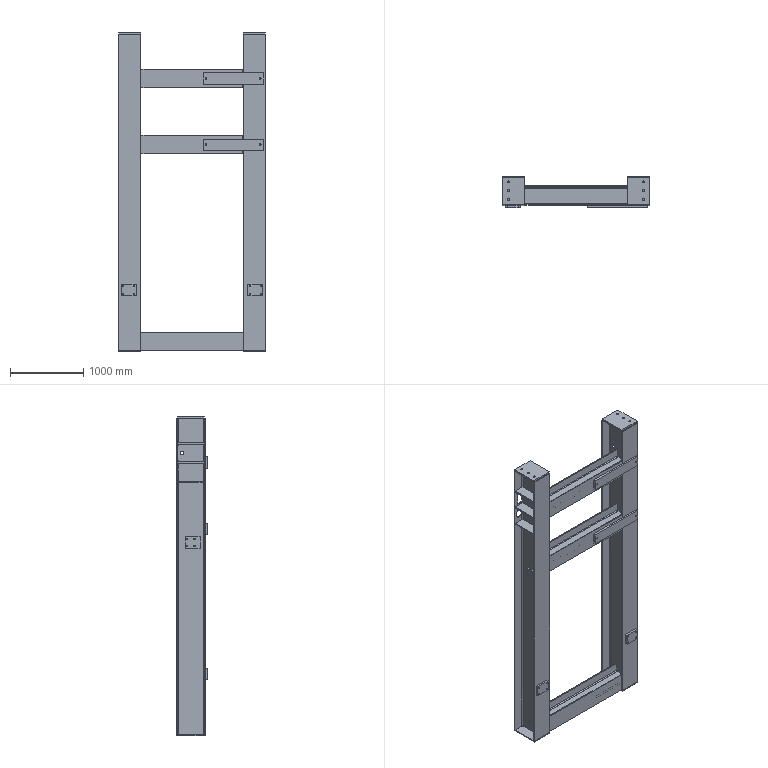Part | SolidWorks | 20 solids | 262 faces | box 1990 x 420 x 4350 mm | volume 182192599 mm3 | plane 187 | cylinder 75 | commonest cylinder face diameters 26 x23 17.5 x16 27.5 x12 16.667 x8 21 x8 51 x4